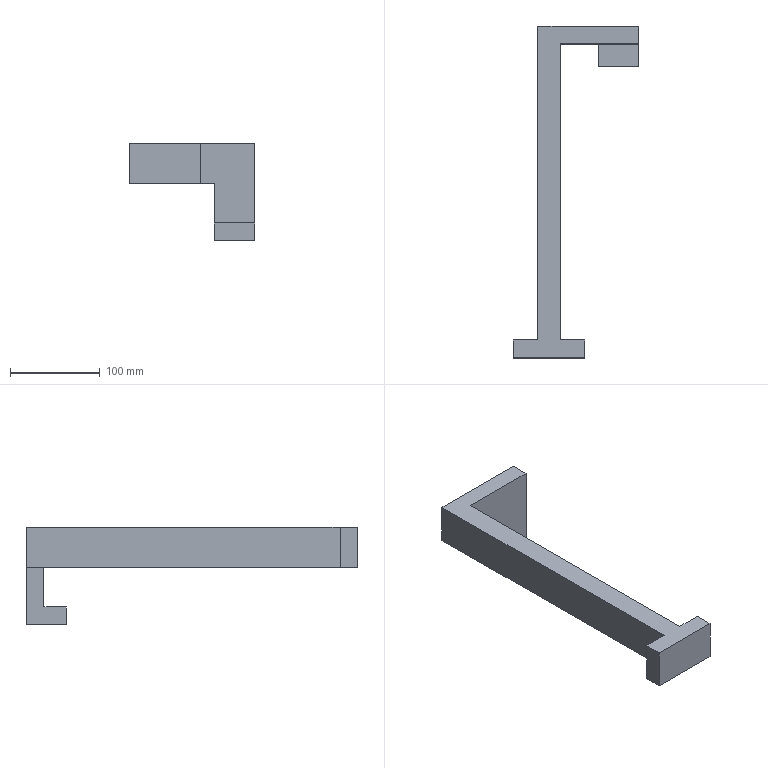Part | STEP file | Stopper | 1 solid | 16 faces | box 140 x 370 x 109 mm | volume 624600 mm3 | plane 16
STEP:
#1=CARTESIAN_POINT('',(0.,0.,0.));
#2=DIRECTION('',(0.,0.,1.));
#3=DIRECTION('',(1.,0.,0.));
#4=AXIS2_PLACEMENT_3D('',#1,#2,#3);
#5=CARTESIAN_POINT('',(112.5,-20.,-44.));
#6=VERTEX_POINT('',#5);
#7=CARTESIAN_POINT('',(67.5,-20.,-44.));
#8=VERTEX_POINT('',#7);
#9=CARTESIAN_POINT('',(67.5,-20.,-44.));
#10=DIRECTION('',(-1.,0.,0.));
#11=VECTOR('',#10,1.);
#12=LINE('',#9,#11);
#13=CARTESIAN_POINT('',(112.5,-20.,45.));
#14=DIRECTION('',(0.,1.,0.));
#15=DIRECTION('',(0.,0.,1.));
#16=AXIS2_PLACEMENT_3D('',#13,#14,#15);
#17=PLANE('',#16);
#18=CARTESIAN_POINT('',(-89.,-45.));
#19=DIRECTION('',(0.,-1.));
#20=VECTOR('',#19,1.);
#21=LINE('',#18,#20);
#22=(GEOMETRIC_REPRESENTATION_CONTEXT(2)PARAMETRIC_REPRESENTATION_CONTEXT()REPRESENTATION_CONTEXT('',''));
#23=DEFINITIONAL_REPRESENTATION('',(#21),#22);
#24=PCURVE('',#17,#23);
#25=CARTESIAN_POINT('',(67.5,-45.,-44.));
#26=DIRECTION('',(0.,0.,-1.));
#27=DIRECTION('',(-1.,0.,0.));
#28=AXIS2_PLACEMENT_3D('',#25,#26,#27);
#29=PLANE('',#28);
#30=CARTESIAN_POINT('',(0.,25.));
#31=DIRECTION('',(1.,0.));
#32=VECTOR('',#31,1.);
#33=LINE('',#30,#32);
#34=(GEOMETRIC_REPRESENTATION_CONTEXT(2)PARAMETRIC_REPRESENTATION_CONTEXT()REPRESENTATION_CONTEXT('',''));
#35=DEFINITIONAL_REPRESENTATION('',(#33),#34);
#36=PCURVE('',#29,#35);
#37=SURFACE_CURVE('',#12,(#24,#36),.PCURVE_S1.);
#38=EDGE_CURVE('',#6,#8,#37,.T.);
#39=ORIENTED_EDGE('',*,*,#38,.F.);
#40=CARTESIAN_POINT('',(112.5,-20.,45.));
#41=VERTEX_POINT('',#40);
#42=CARTESIAN_POINT('',(112.5,-20.,45.));
#43=DIRECTION('',(0.,0.,-1.));
#44=VECTOR('',#43,1.);
#45=LINE('',#42,#44);
#46=CARTESIAN_POINT('',(0.,0.));
#47=DIRECTION('',(-1.,0.));
#48=VECTOR('',#47,1.);
#49=LINE('',#46,#48);
#50=(GEOMETRIC_REPRESENTATION_CONTEXT(2)PARAMETRIC_REPRESENTATION_CONTEXT()REPRESENTATION_CONTEXT('',''));
#51=DEFINITIONAL_REPRESENTATION('',(#49),#50);
#52=PCURVE('',#17,#51);
#53=CARTESIAN_POINT('',(112.5,-20.,45.));
#54=DIRECTION('',(1.,0.,0.));
#55=DIRECTION('',(0.,0.,-1.));
#56=AXIS2_PLACEMENT_3D('',#53,#54,#55);
#57=PLANE('',#56);
#58=CARTESIAN_POINT('',(0.,0.));
#59=DIRECTION('',(1.,0.));
#60=VECTOR('',#59,1.);
#61=LINE('',#58,#60);
#62=(GEOMETRIC_REPRESENTATION_CONTEXT(2)PARAMETRIC_REPRESENTATION_CONTEXT()REPRESENTATION_CONTEXT('',''));
#63=DEFINITIONAL_REPRESENTATION('',(#61),#62);
#64=PCURVE('',#57,#63);
#65=SURFACE_CURVE('',#45,(#52,#64),.PCURVE_S1.);
#66=EDGE_CURVE('',#41,#6,#65,.T.);
#67=ORIENTED_EDGE('',*,*,#66,.F.);
#68=CARTESIAN_POINT('',(25.,-20.,45.));
#69=VERTEX_POINT('',#68);
#70=CARTESIAN_POINT('',(112.5,-20.,45.));
#71=DIRECTION('',(-1.,0.,0.));
#72=VECTOR('',#71,1.);
#73=LINE('',#70,#72);
#74=CARTESIAN_POINT('',(0.,0.));
#75=DIRECTION('',(0.,-1.));
#76=VECTOR('',#75,1.);
#77=LINE('',#74,#76);
#78=(GEOMETRIC_REPRESENTATION_CONTEXT(2)PARAMETRIC_REPRESENTATION_CONTEXT()REPRESENTATION_CONTEXT('',''));
#79=DEFINITIONAL_REPRESENTATION('',(#77),#78);
#80=PCURVE('',#17,#79);
#81=CARTESIAN_POINT('',(0.,0.,45.));
#82=DIRECTION('',(0.,0.,1.));
#83=DIRECTION('',(1.,0.,0.));
#84=AXIS2_PLACEMENT_3D('',#81,#82,#83);
#85=PLANE('',#84);
#86=CARTESIAN_POINT('',(112.5,-20.));
#87=DIRECTION('',(-1.,0.));
#88=VECTOR('',#87,1.);
#89=LINE('',#86,#88);
#90=(GEOMETRIC_REPRESENTATION_CONTEXT(2)PARAMETRIC_REPRESENTATION_CONTEXT()REPRESENTATION_CONTEXT('',''));
#91=DEFINITIONAL_REPRESENTATION('',(#89),#90);
#92=PCURVE('',#85,#91);
#93=SURFACE_CURVE('',#73,(#80,#92),.PCURVE_S1.);
#94=EDGE_CURVE('',#41,#69,#93,.T.);
#95=ORIENTED_EDGE('',*,*,#94,.T.);
#96=CARTESIAN_POINT('',(25.,-20.,0.));
#97=VERTEX_POINT('',#96);
#98=CARTESIAN_POINT('',(25.,-20.,45.));
#99=DIRECTION('',(0.,0.,-1.));
#100=VECTOR('',#99,1.);
#101=LINE('',#98,#100);
#102=CARTESIAN_POINT('',(0.,-87.5));
#103=DIRECTION('',(-1.,0.));
#104=VECTOR('',#103,1.);
#105=LINE('',#102,#104);
#106=(GEOMETRIC_REPRESENTATION_CONTEXT(2)PARAMETRIC_REPRESENTATION_CONTEXT()REPRESENTATION_CONTEXT('',''));
#107=DEFINITIONAL_REPRESENTATION('',(#105),#106);
#108=PCURVE('',#17,#107);
#109=CARTESIAN_POINT('',(25.,-350.,45.));
#110=DIRECTION('',(-1.,0.,0.));
#111=DIRECTION('',(0.,0.,1.));
#112=AXIS2_PLACEMENT_3D('',#109,#110,#111);
#113=PLANE('',#112);
#114=CARTESIAN_POINT('',(0.,330.));
#115=DIRECTION('',(-1.,0.));
#116=VECTOR('',#115,1.);
#117=LINE('',#114,#116);
#118=(GEOMETRIC_REPRESENTATION_CONTEXT(2)PARAMETRIC_REPRESENTATION_CONTEXT()REPRESENTATION_CONTEXT('',''));
#119=DEFINITIONAL_REPRESENTATION('',(#117),#118);
#120=PCURVE('',#113,#119);
#121=SURFACE_CURVE('',#101,(#108,#120),.PCURVE_S1.);
#122=EDGE_CURVE('',#69,#97,#121,.T.);
#123=ORIENTED_EDGE('',*,*,#122,.T.);
#124=CARTESIAN_POINT('',(67.5,-20.,0.));
#125=VERTEX_POINT('',#124);
#126=CARTESIAN_POINT('',(112.5,-20.,0.));
#127=DIRECTION('',(-1.,0.,0.));
#128=VECTOR('',#127,1.);
#129=LINE('',#126,#128);
#130=CARTESIAN_POINT('',(-45.,0.));
#131=DIRECTION('',(0.,-1.));
#132=VECTOR('',#131,1.);
#133=LINE('',#130,#132);
#134=(GEOMETRIC_REPRESENTATION_CONTEXT(2)PARAMETRIC_REPRESENTATION_CONTEXT()REPRESENTATION_CONTEXT('',''));
#135=DEFINITIONAL_REPRESENTATION('',(#133),#134);
#136=PCURVE('',#17,#135);
#137=CARTESIAN_POINT('',(0.,0.,0.));
#138=DIRECTION('',(0.,0.,1.));
#139=DIRECTION('',(1.,0.,0.));
#140=AXIS2_PLACEMENT_3D('',#137,#138,#139);
#141=PLANE('',#140);
#142=CARTESIAN_POINT('',(112.5,-20.));
#143=DIRECTION('',(-1.,0.));
#144=VECTOR('',#143,1.);
#145=LINE('',#142,#144);
#146=(GEOMETRIC_REPRESENTATION_CONTEXT(2)PARAMETRIC_REPRESENTATION_CONTEXT()REPRESENTATION_CONTEXT('',''));
#147=DEFINITIONAL_REPRESENTATION('',(#145),#146);
#148=PCURVE('',#141,#147);
#149=SURFACE_CURVE('',#129,(#136,#148),.PCURVE_S1.);
#150=EDGE_CURVE('',#125,#97,#149,.T.);
#151=ORIENTED_EDGE('',*,*,#150,.F.);
#152=CARTESIAN_POINT('',(67.5,-20.,-64.));
#153=DIRECTION('',(0.,0.,1.));
#154=VECTOR('',#153,1.);
#155=LINE('',#152,#154);
#156=CARTESIAN_POINT('',(-109.,-45.));
#157=DIRECTION('',(1.,0.));
#158=VECTOR('',#157,1.);
#159=LINE('',#156,#158);
#160=(GEOMETRIC_REPRESENTATION_CONTEXT(2)PARAMETRIC_REPRESENTATION_CONTEXT()REPRESENTATION_CONTEXT('',''));
#161=DEFINITIONAL_REPRESENTATION('',(#159),#160);
#162=PCURVE('',#17,#161);
#163=CARTESIAN_POINT('',(67.5,0.,-64.));
#164=DIRECTION('',(1.,0.,0.));
#165=DIRECTION('',(0.,0.,-1.));
#166=AXIS2_PLACEMENT_3D('',#163,#164,#165);
#167=PLANE('',#166);
#168=CARTESIAN_POINT('',(0.,-20.));
#169=DIRECTION('',(-1.,0.));
#170=VECTOR('',#169,1.);
#171=LINE('',#168,#170);
#172=(GEOMETRIC_REPRESENTATION_CONTEXT(2)PARAMETRIC_REPRESENTATION_CONTEXT()REPRESENTATION_CONTEXT('',''));
#173=DEFINITIONAL_REPRESENTATION('',(#171),#172);
#174=PCURVE('',#167,#173);
#175=SURFACE_CURVE('',#155,(#162,#174),.PCURVE_S1.);
#176=EDGE_CURVE('',#8,#125,#175,.T.);
#177=ORIENTED_EDGE('',*,*,#176,.F.);
#178=EDGE_LOOP('',(#39,#67,#95,#123,#151,#177));
#179=FACE_BOUND('',#178,.T.);
#180=ADVANCED_FACE('',(#179),#17,.F.);
#181=CARTESIAN_POINT('',(67.5,0.,0.));
#182=VERTEX_POINT('',#181);
#183=CARTESIAN_POINT('',(67.5,0.,0.));
#184=DIRECTION('',(0.,1.,0.));
#185=VECTOR('',#184,1.);
#186=LINE('',#183,#185);
#187=CARTESIAN_POINT('',(67.5,0.));
#188=DIRECTION('',(0.,1.));
#189=VECTOR('',#188,1.);
#190=LINE('',#187,#189);
#191=(GEOMETRIC_REPRESENTATION_CONTEXT(2)PARAMETRIC_REPRESENTATION_CONTEXT()REPRESENTATION_CONTEXT('',''));
#192=DEFINITIONAL_REPRESENTATION('',(#190),#191);
#193=PCURVE('',#141,#192);
#194=CARTESIAN_POINT('',(-64.,0.));
#195=DIRECTION('',(0.,1.));
#196=VECTOR('',#195,1.);
#197=LINE('',#194,#196);
#198=(GEOMETRIC_REPRESENTATION_CONTEXT(2)PARAMETRIC_REPRESENTATION_CONTEXT()REPRESENTATION_CONTEXT('',''));
#199=DEFINITIONAL_REPRESENTATION('',(#197),#198);
#200=PCURVE('',#167,#199);
#201=SURFACE_CURVE('',#186,(#193,#200),.PCURVE_S1.);
#202=EDGE_CURVE('',#125,#182,#201,.T.);
#203=ORIENTED_EDGE('',*,*,#202,.F.);
#204=ORIENTED_EDGE('',*,*,#150,.T.);
#205=CARTESIAN_POINT('',(25.,-350.,0.));
#206=VERTEX_POINT('',#205);
#207=CARTESIAN_POINT('',(25.,-350.,0.));
#208=DIRECTION('',(0.,1.,0.));
#209=VECTOR('',#208,1.);
#210=LINE('',#207,#209);
#211=CARTESIAN_POINT('',(25.,-350.));
#212=DIRECTION('',(0.,1.));
#213=VECTOR('',#212,1.);
#214=LINE('',#211,#213);
#215=(GEOMETRIC_REPRESENTATION_CONTEXT(2)PARAMETRIC_REPRESENTATION_CONTEXT()REPRESENTATION_CONTEXT('',''));
#216=DEFINITIONAL_REPRESENTATION('',(#214),#215);
#217=PCURVE('',#141,#216);
#218=CARTESIAN_POINT('',(-45.,0.));
#219=DIRECTION('',(0.,1.));
#220=VECTOR('',#219,1.);
#221=LINE('',#218,#220);
#222=(GEOMETRIC_REPRESENTATION_CONTEXT(2)PARAMETRIC_REPRESENTATION_CONTEXT()REPRESENTATION_CONTEXT('',''));
#223=DEFINITIONAL_REPRESENTATION('',(#221),#222);
#224=PCURVE('',#113,#223);
#225=SURFACE_CURVE('',#210,(#217,#224),.PCURVE_S1.);
#226=EDGE_CURVE('',#206,#97,#225,.T.);
#227=ORIENTED_EDGE('',*,*,#226,.F.);
#228=CARTESIAN_POINT('',(52.5,-350.,0.));
#229=VERTEX_POINT('',#228);
#230=CARTESIAN_POINT('',(52.5,-350.,0.));
#231=DIRECTION('',(-1.,0.,0.));
#232=VECTOR('',#231,1.);
#233=LINE('',#230,#232);
#234=CARTESIAN_POINT('',(52.5,-350.));
#235=DIRECTION('',(-1.,0.));
#236=VECTOR('',#235,1.);
#237=LINE('',#234,#236);
#238=(GEOMETRIC_REPRESENTATION_CONTEXT(2)PARAMETRIC_REPRESENTATION_CONTEXT()REPRESENTATION_CONTEXT('',''));
#239=DEFINITIONAL_REPRESENTATION('',(#237),#238);
#240=PCURVE('',#141,#239);
#241=CARTESIAN_POINT('',(52.5,-350.,45.));
#242=DIRECTION('',(0.,-1.,0.));
#243=DIRECTION('',(0.,0.,-1.));
#244=AXIS2_PLACEMENT_3D('',#241,#242,#243);
#245=PLANE('',#244);
#246=CARTESIAN_POINT('',(45.,0.));
#247=DIRECTION('',(0.,-1.));
#248=VECTOR('',#247,1.);
#249=LINE('',#246,#248);
#250=(GEOMETRIC_REPRESENTATION_CONTEXT(2)PARAMETRIC_REPRESENTATION_CONTEXT()REPRESENTATION_CONTEXT('',''));
#251=DEFINITIONAL_REPRESENTATION('',(#249),#250);
#252=PCURVE('',#245,#251);
#253=SURFACE_CURVE('',#233,(#240,#252),.PCURVE_S1.);
#254=EDGE_CURVE('',#229,#206,#253,.T.);
#255=ORIENTED_EDGE('',*,*,#254,.F.);
#256=CARTESIAN_POINT('',(52.5,-370.,0.));
#257=VERTEX_POINT('',#256);
#258=CARTESIAN_POINT('',(52.5,-370.,0.));
#259=DIRECTION('',(0.,1.,0.));
#260=VECTOR('',#259,1.);
#261=LINE('',#258,#260);
#262=CARTESIAN_POINT('',(52.5,-370.));
#263=DIRECTION('',(0.,1.));
#264=VECTOR('',#263,1.);
#265=LINE('',#262,#264);
#266=(GEOMETRIC_REPRESENTATION_CONTEXT(2)PARAMETRIC_REPRESENTATION_CONTEXT()REPRESENTATION_CONTEXT('',''));
#267=DEFINITIONAL_REPRESENTATION('',(#265),#266);
#268=PCURVE('',#141,#267);
#269=CARTESIAN_POINT('',(52.5,-370.,45.));
#270=DIRECTION('',(-1.,0.,0.));
#271=DIRECTION('',(0.,-1.,0.));
#272=AXIS2_PLACEMENT_3D('',#269,#270,#271);
#273=PLANE('',#272);
#274=CARTESIAN_POINT('',(0.,-45.));
#275=DIRECTION('',(-1.,0.));
#276=VECTOR('',#275,1.);
#277=LINE('',#274,#276);
#278=(GEOMETRIC_REPRESENTATION_CONTEXT(2)PARAMETRIC_REPRESENTATION_CONTEXT()REPRESENTATION_CONTEXT('',''));
#279=DEFINITIONAL_REPRESENTATION('',(#277),#278);
#280=PCURVE('',#273,#279);
#281=SURFACE_CURVE('',#261,(#268,#280),.PCURVE_S1.);
#282=EDGE_CURVE('',#257,#229,#281,.T.);
#283=ORIENTED_EDGE('',*,*,#282,.F.);
#284=CARTESIAN_POINT('',(-27.5,-370.,0.));
#285=VERTEX_POINT('',#284);
#286=CARTESIAN_POINT('',(-27.5,-370.,0.));
#287=DIRECTION('',(1.,0.,0.));
#288=VECTOR('',#287,1.);
#289=LINE('',#286,#288);
#290=CARTESIAN_POINT('',(-27.5,-370.));
#291=DIRECTION('',(1.,0.));
#292=VECTOR('',#291,1.);
#293=LINE('',#290,#292);
#294=(GEOMETRIC_REPRESENTATION_CONTEXT(2)PARAMETRIC_REPRESENTATION_CONTEXT()REPRESENTATION_CONTEXT('',''));
#295=DEFINITIONAL_REPRESENTATION('',(#293),#294);
#296=PCURVE('',#141,#295);
#297=CARTESIAN_POINT('',(-27.5,-370.,45.));
#298=DIRECTION('',(0.,1.,0.));
#299=DIRECTION('',(0.,0.,1.));
#300=AXIS2_PLACEMENT_3D('',#297,#298,#299);
#301=PLANE('',#300);
#302=CARTESIAN_POINT('',(-45.,0.));
#303=DIRECTION('',(0.,1.));
#304=VECTOR('',#303,1.);
#305=LINE('',#302,#304);
#306=(GEOMETRIC_REPRESENTATION_CONTEXT(2)PARAMETRIC_REPRESENTATION_CONTEXT()REPRESENTATION_CONTEXT('',''));
#307=DEFINITIONAL_REPRESENTATION('',(#305),#306);
#308=PCURVE('',#301,#307);
#309=SURFACE_CURVE('',#289,(#296,#308),.PCURVE_S1.);
#310=EDGE_CURVE('',#285,#257,#309,.T.);
#311=ORIENTED_EDGE('',*,*,#310,.F.);
#312=CARTESIAN_POINT('',(-27.5,-350.,0.));
#313=VERTEX_POINT('',#312);
#314=CARTESIAN_POINT('',(-27.5,-350.,0.));
#315=DIRECTION('',(0.,-1.,0.));
#316=VECTOR('',#315,1.);
#317=LINE('',#314,#316);
#318=CARTESIAN_POINT('',(-27.5,-350.));
#319=DIRECTION('',(0.,-1.));
#320=VECTOR('',#319,1.);
#321=LINE('',#318,#320);
#322=(GEOMETRIC_REPRESENTATION_CONTEXT(2)PARAMETRIC_REPRESENTATION_CONTEXT()REPRESENTATION_CONTEXT('',''));
#323=DEFINITIONAL_REPRESENTATION('',(#321),#322);
#324=PCURVE('',#141,#323);
#325=CARTESIAN_POINT('',(-27.5,-350.,45.));
#326=DIRECTION('',(1.,0.,0.));
#327=DIRECTION('',(0.,1.,0.));
#328=AXIS2_PLACEMENT_3D('',#325,#326,#327);
#329=PLANE('',#328);
#330=CARTESIAN_POINT('',(0.,-45.));
#331=DIRECTION('',(-1.,0.));
#332=VECTOR('',#331,1.);
#333=LINE('',#330,#332);
#334=(GEOMETRIC_REPRESENTATION_CONTEXT(2)PARAMETRIC_REPRESENTATION_CONTEXT()REPRESENTATION_CONTEXT('',''));
#335=DEFINITIONAL_REPRESENTATION('',(#333),#334);
#336=PCURVE('',#329,#335);
#337=SURFACE_CURVE('',#317,(#324,#336),.PCURVE_S1.);
#338=EDGE_CURVE('',#313,#285,#337,.T.);
#339=ORIENTED_EDGE('',*,*,#338,.F.);
#340=CARTESIAN_POINT('',(0.,-350.,0.));
#341=VERTEX_POINT('',#340);
#342=CARTESIAN_POINT('',(0.,-350.,0.));
#343=DIRECTION('',(-1.,0.,0.));
#344=VECTOR('',#343,1.);
#345=LINE('',#342,#344);
#346=CARTESIAN_POINT('',(0.,-350.));
#347=DIRECTION('',(-1.,0.));
#348=VECTOR('',#347,1.);
#349=LINE('',#346,#348);
#350=(GEOMETRIC_REPRESENTATION_CONTEXT(2)PARAMETRIC_REPRESENTATION_CONTEXT()REPRESENTATION_CONTEXT('',''));
#351=DEFINITIONAL_REPRESENTATION('',(#349),#350);
#352=PCURVE('',#141,#351);
#353=CARTESIAN_POINT('',(0.,-350.,45.));
#354=DIRECTION('',(0.,-1.,0.));
#355=DIRECTION('',(0.,0.,-1.));
#356=AXIS2_PLACEMENT_3D('',#353,#354,#355);
#357=PLANE('',#356);
#358=CARTESIAN_POINT('',(45.,0.));
#359=DIRECTION('',(0.,-1.));
#360=VECTOR('',#359,1.);
#361=LINE('',#358,#360);
#362=(GEOMETRIC_REPRESENTATION_CONTEXT(2)PARAMETRIC_REPRESENTATION_CONTEXT()REPRESENTATION_CONTEXT('',''));
#363=DEFINITIONAL_REPRESENTATION('',(#361),#362);
#364=PCURVE('',#357,#363);
#365=SURFACE_CURVE('',#345,(#352,#364),.PCURVE_S1.);
#366=EDGE_CURVE('',#341,#313,#365,.T.);
#367=ORIENTED_EDGE('',*,*,#366,.F.);
#368=CARTESIAN_POINT('',(0.,0.,0.));
#369=VERTEX_POINT('',#368);
#370=CARTESIAN_POINT('',(0.,0.,0.));
#371=DIRECTION('',(0.,-1.,0.));
#372=VECTOR('',#371,1.);
#373=LINE('',#370,#372);
#374=CARTESIAN_POINT('',(0.,0.));
#375=DIRECTION('',(0.,-1.));
#376=VECTOR('',#375,1.);
#377=LINE('',#374,#376);
#378=(GEOMETRIC_REPRESENTATION_CONTEXT(2)PARAMETRIC_REPRESENTATION_CONTEXT()REPRESENTATION_CONTEXT('',''));
#379=DEFINITIONAL_REPRESENTATION('',(#377),#378);
#380=PCURVE('',#141,#379);
#381=CARTESIAN_POINT('',(0.,0.,45.));
#382=DIRECTION('',(1.,0.,0.));
#383=DIRECTION('',(0.,1.,0.));
#384=AXIS2_PLACEMENT_3D('',#381,#382,#383);
#385=PLANE('',#384);
#386=CARTESIAN_POINT('',(0.,-45.));
#387=DIRECTION('',(-1.,0.));
#388=VECTOR('',#387,1.);
#389=LINE('',#386,#388);
#390=(GEOMETRIC_REPRESENTATION_CONTEXT(2)PARAMETRIC_REPRESENTATION_CONTEXT()REPRESENTATION_CONTEXT('',''));
#391=DEFINITIONAL_REPRESENTATION('',(#389),#390);
#392=PCURVE('',#385,#391);
#393=SURFACE_CURVE('',#373,(#380,#392),.PCURVE_S1.);
#394=EDGE_CURVE('',#369,#341,#393,.T.);
#395=ORIENTED_EDGE('',*,*,#394,.F.);
#396=CARTESIAN_POINT('',(25.,0.,0.));
#397=DIRECTION('',(-1.,0.,0.));
#398=VECTOR('',#397,1.);
#399=LINE('',#396,#398);
#400=CARTESIAN_POINT('',(25.,0.));
#401=DIRECTION('',(-1.,0.));
#402=VECTOR('',#401,1.);
#403=LINE('',#400,#402);
#404=(GEOMETRIC_REPRESENTATION_CONTEXT(2)PARAMETRIC_REPRESENTATION_CONTEXT()REPRESENTATION_CONTEXT('',''));
#405=DEFINITIONAL_REPRESENTATION('',(#403),#404);
#406=PCURVE('',#141,#405);
#407=CARTESIAN_POINT('',(25.,0.,45.));
#408=DIRECTION('',(0.,-1.,0.));
#409=DIRECTION('',(1.,0.,0.));
#410=AXIS2_PLACEMENT_3D('',#407,#408,#409);
#411=PLANE('',#410);
#412=CARTESIAN_POINT('',(0.,-45.));
#413=DIRECTION('',(-1.,0.));
#414=VECTOR('',#413,1.);
#415=LINE('',#412,#414);
#416=(GEOMETRIC_REPRESENTATION_CONTEXT(2)PARAMETRIC_REPRESENTATION_CONTEXT()REPRESENTATION_CONTEXT('',''));
#417=DEFINITIONAL_REPRESENTATION('',(#415),#416);
#418=PCURVE('',#411,#417);
#419=SURFACE_CURVE('',#399,(#406,#418),.PCURVE_S1.);
#420=EDGE_CURVE('',#182,#369,#419,.T.);
#421=ORIENTED_EDGE('',*,*,#420,.F.);
#422=EDGE_LOOP('',(#203,#204,#227,#255,#283,#311,#339,#367,#395,#421));
#423=FACE_BOUND('',#422,.T.);
#424=ADVANCED_FACE('',(#423),#141,.F.);
#425=ORIENTED_EDGE('',*,*,#122,.F.);
#426=CARTESIAN_POINT('',(25.,-350.,45.));
#427=VERTEX_POINT('',#426);
#428=CARTESIAN_POINT('',(25.,-350.,45.));
#429=DIRECTION('',(0.,1.,0.));
#430=VECTOR('',#429,1.);
#431=LINE('',#428,#430);
#432=CARTESIAN_POINT('',(0.,0.));
#433=DIRECTION('',(0.,1.));
#434=VECTOR('',#433,1.);
#435=LINE('',#432,#434);
#436=(GEOMETRIC_REPRESENTATION_CONTEXT(2)PARAMETRIC_REPRESENTATION_CONTEXT()REPRESENTATION_CONTEXT('',''));
#437=DEFINITIONAL_REPRESENTATION('',(#435),#436);
#438=PCURVE('',#113,#437);
#439=CARTESIAN_POINT('',(25.,-350.));
#440=DIRECTION('',(0.,1.));
#441=VECTOR('',#440,1.);
#442=LINE('',#439,#441);
#443=(GEOMETRIC_REPRESENTATION_CONTEXT(2)PARAMETRIC_REPRESENTATION_CONTEXT()REPRESENTATION_CONTEXT('',''));
#444=DEFINITIONAL_REPRESENTATION('',(#442),#443);
#445=PCURVE('',#85,#444);
#446=SURFACE_CURVE('',#431,(#438,#445),.PCURVE_S1.);
#447=EDGE_CURVE('',#427,#69,#446,.T.);
#448=ORIENTED_EDGE('',*,*,#447,.F.);
#449=CARTESIAN_POINT('',(25.,-350.,45.));
#450=DIRECTION('',(0.,0.,-1.));
#451=VECTOR('',#450,1.);
#452=LINE('',#449,#451);
#453=CARTESIAN_POINT('',(0.,0.));
#454=DIRECTION('',(-1.,0.));
#455=VECTOR('',#454,1.);
#456=LINE('',#453,#455);
#457=(GEOMETRIC_REPRESENTATION_CONTEXT(2)PARAMETRIC_REPRESENTATION_CONTEXT()REPRESENTATION_CONTEXT('',''));
#458=DEFINITIONAL_REPRESENTATION('',(#456),#457);
#459=PCURVE('',#113,#458);
#460=CARTESIAN_POINT('',(0.,-27.5));
#461=DIRECTION('',(1.,0.));
#462=VECTOR('',#461,1.);
#463=LINE('',#460,#462);
#464=(GEOMETRIC_REPRESENTATION_CONTEXT(2)PARAMETRIC_REPRESENTATION_CONTEXT()REPRESENTATION_CONTEXT('',''));
#465=DEFINITIONAL_REPRESENTATION('',(#463),#464);
#466=PCURVE('',#245,#465);
#467=SURFACE_CURVE('',#452,(#459,#466),.PCURVE_S1.);
#468=EDGE_CURVE('',#427,#206,#467,.T.);
#469=ORIENTED_EDGE('',*,*,#468,.T.);
#470=ORIENTED_EDGE('',*,*,#226,.T.);
#471=EDGE_LOOP('',(#425,#448,#469,#470));
#472=FACE_BOUND('',#471,.T.);
#473=ADVANCED_FACE('',(#472),#113,.F.);
#474=CARTESIAN_POINT('',(112.5,0.,-64.));
#475=VERTEX_POINT('',#474);
#476=CARTESIAN_POINT('',(112.5,0.,45.));
#477=VERTEX_POINT('',#476);
#478=CARTESIAN_POINT('',(112.5,0.,45.));
#479=DIRECTION('',(0.,0.,1.));
#480=VECTOR('',#479,1.);
#481=LINE('',#478,#480);
#482=CARTESIAN_POINT('',(87.5,0.));
#483=DIRECTION('',(0.,1.));
#484=VECTOR('',#483,1.);
#485=LINE('',#482,#484);
#486=(GEOMETRIC_REPRESENTATION_CONTEXT(2)PARAMETRIC_REPRESENTATION_CONTEXT()REPRESENTATION_CONTEXT('',''));
#487=DEFINITIONAL_REPRESENTATION('',(#485),#486);
#488=PCURVE('',#411,#487);
#489=CARTESIAN_POINT('',(0.,20.));
#490=DIRECTION('',(-1.,0.));
#491=VECTOR('',#490,1.);
#492=LINE('',#489,#491);
#493=(GEOMETRIC_REPRESENTATION_CONTEXT(2)PARAMETRIC_REPRESENTATION_CONTEXT()REPRESENTATION_CONTEXT('',''));
#494=DEFINITIONAL_REPRESENTATION('',(#492),#493);
#495=PCURVE('',#57,#494);
#496=SURFACE_CURVE('',#481,(#488,#495),.PCURVE_S1.);
#497=EDGE_CURVE('',#475,#477,#496,.T.);
#498=ORIENTED_EDGE('',*,*,#497,.F.);
#499=CARTESIAN_POINT('',(67.5,0.,-64.));
#500=VERTEX_POINT('',#499);
#501=CARTESIAN_POINT('',(112.5,0.,-64.));
#502=DIRECTION('',(1.,0.,0.));
#503=VECTOR('',#502,1.);
#504=LINE('',#501,#503);
#505=CARTESIAN_POINT('',(87.5,-109.));
#506=DIRECTION('',(1.,0.));
#507=VECTOR('',#506,1.);
#508=LINE('',#505,#507);
#509=(GEOMETRIC_REPRESENTATION_CONTEXT(2)PARAMETRIC_REPRESENTATION_CONTEXT()REPRESENTATION_CONTEXT('',''));
#510=DEFINITIONAL_REPRESENTATION('',(#508),#509);
#511=PCURVE('',#411,#510);
#512=CARTESIAN_POINT('',(112.5,-20.,-64.));
#513=DIRECTION('',(0.,0.,-1.));
#514=DIRECTION('',(-1.,0.,0.));
#515=AXIS2_PLACEMENT_3D('',#512,#513,#514);
#516=PLANE('',#515);
#517=CARTESIAN_POINT('',(0.,20.));
#518=DIRECTION('',(-1.,0.));
#519=VECTOR('',#518,1.);
#520=LINE('',#517,#519);
#521=(GEOMETRIC_REPRESENTATION_CONTEXT(2)PARAMETRIC_REPRESENTATION_CONTEXT()REPRESENTATION_CONTEXT('',''));
#522=DEFINITIONAL_REPRESENTATION('',(#520),#521);
#523=PCURVE('',#516,#522);
#524=SURFACE_CURVE('',#504,(#511,#523),.PCURVE_S1.);
#525=EDGE_CURVE('',#500,#475,#524,.T.);
#526=ORIENTED_EDGE('',*,*,#525,.F.);
#527=CARTESIAN_POINT('',(67.5,0.,-64.));
#528=DIRECTION('',(0.,0.,1.));
#529=VECTOR('',#528,1.);
#530=LINE('',#527,#529);
#531=CARTESIAN_POINT('',(42.5,-109.));
#532=DIRECTION('',(0.,1.));
#533=VECTOR('',#532,1.);
#534=LINE('',#531,#533);
#535=(GEOMETRIC_REPRESENTATION_CONTEXT(2)PARAMETRIC_REPRESENTATION_CONTEXT()REPRESENTATION_CONTEXT('',''));
#536=DEFINITIONAL_REPRESENTATION('',(#534),#535);
#537=PCURVE('',#411,#536);
#538=CARTESIAN_POINT('',(0.,0.));
#539=DIRECTION('',(-1.,0.));
#540=VECTOR('',#539,1.);
#541=LINE('',#538,#540);
#542=(GEOMETRIC_REPRESENTATION_CONTEXT(2)PARAMETRIC_REPRESENTATION_CONTEXT()REPRESENTATION_CONTEXT('',''));
#543=DEFINITIONAL_REPRESENTATION('',(#541),#542);
#544=PCURVE('',#167,#543);
#545=SURFACE_CURVE('',#530,(#537,#544),.PCURVE_S1.);
#546=EDGE_CURVE('',#500,#182,#545,.T.);
#547=ORIENTED_EDGE('',*,*,#546,.T.);
#548=ORIENTED_EDGE('',*,*,#420,.T.);
#549=CARTESIAN_POINT('',(0.,0.,45.));
#550=VERTEX_POINT('',#549);
#551=CARTESIAN_POINT('',(0.,0.,45.));
#552=DIRECTION('',(0.,0.,-1.));
#553=VECTOR('',#552,1.);
#554=LINE('',#551,#553);
#555=CARTESIAN_POINT('',(-25.,0.));
#556=DIRECTION('',(0.,-1.));
#557=VECTOR('',#556,1.);
#558=LINE('',#555,#557);
#559=(GEOMETRIC_REPRESENTATION_CONTEXT(2)PARAMETRIC_REPRESENTATION_CONTEXT()REPRESENTATION_CONTEXT('',''));
#560=DEFINITIONAL_REPRESENTATION('',(#558),#559);
#561=PCURVE('',#411,#560);
#562=CARTESIAN_POINT('',(0.,0.));
#563=DIRECTION('',(0.,-1.));
#564=VECTOR('',#563,1.);
#565=LINE('',#562,#564);
#566=(GEOMETRIC_REPRESENTATION_CONTEXT(2)PARAMETRIC_REPRESENTATION_CONTEXT()REPRESENTATION_CONTEXT('',''));
#567=DEFINITIONAL_REPRESENTATION('',(#565),#566);
#568=PCURVE('',#385,#567);
#569=SURFACE_CURVE('',#554,(#561,#568),.PCURVE_S1.);
#570=EDGE_CURVE('',#550,#369,#569,.T.);
#571=ORIENTED_EDGE('',*,*,#570,.F.);
#572=CARTESIAN_POINT('',(25.,0.,45.));
#573=DIRECTION('',(-1.,0.,0.));
#574=VECTOR('',#573,1.);
#575=LINE('',#572,#574);
#576=CARTESIAN_POINT('',(0.,0.));
#577=DIRECTION('',(-1.,0.));
#578=VECTOR('',#577,1.);
#579=LINE('',#576,#578);
#580=(GEOMETRIC_REPRESENTATION_CONTEXT(2)PARAMETRIC_REPRESENTATION_CONTEXT()REPRESENTATION_CONTEXT('',''));
#581=DEFINITIONAL_REPRESENTATION('',(#579),#580);
#582=PCURVE('',#411,#581);
#583=CARTESIAN_POINT('',(25.,0.));
#584=DIRECTION('',(-1.,0.));
#585=VECTOR('',#584,1.);
#586=LINE('',#583,#585);
#587=(GEOMETRIC_REPRESENTATION_CONTEXT(2)PARAMETRIC_REPRESENTATION_CONTEXT()REPRESENTATION_CONTEXT('',''));
#588=DEFINITIONAL_REPRESENTATION('',(#586),#587);
#589=PCURVE('',#85,#588);
#590=SURFACE_CURVE('',#575,(#582,#589),.PCURVE_S1.);
#591=EDGE_CURVE('',#477,#550,#590,.T.);
#592=ORIENTED_EDGE('',*,*,#591,.F.);
#593=EDGE_LOOP('',(#498,#526,#547,#548,#571,#592));
#594=FACE_BOUND('',#593,.T.);
#595=ADVANCED_FACE('',(#594),#411,.F.);
#596=ORIENTED_EDGE('',*,*,#394,.T.);
#597=CARTESIAN_POINT('',(0.,-350.,45.));
#598=VERTEX_POINT('',#597);
#599=CARTESIAN_POINT('',(0.,-350.,45.));
#600=DIRECTION('',(0.,0.,-1.));
#601=VECTOR('',#600,1.);
#602=LINE('',#599,#601);
#603=CARTESIAN_POINT('',(-350.,0.));
#604=DIRECTION('',(0.,-1.));
#605=VECTOR('',#604,1.);
#606=LINE('',#603,#605);
#607=(GEOMETRIC_REPRESENTATION_CONTEXT(2)PARAMETRIC_REPRESENTATION_CONTEXT()REPRESENTATION_CONTEXT('',''));
#608=DEFINITIONAL_REPRESENTATION('',(#606),#607);
#609=PCURVE('',#385,#608);
#610=CARTESIAN_POINT('',(0.,0.));
#611=DIRECTION('',(1.,0.));
#612=VECTOR('',#611,1.);
#613=LINE('',#610,#612);
#614=(GEOMETRIC_REPRESENTATION_CONTEXT(2)PARAMETRIC_REPRESENTATION_CONTEXT()REPRESENTATION_CONTEXT('',''));
#615=DEFINITIONAL_REPRESENTATION('',(#613),#614);
#616=PCURVE('',#357,#615);
#617=SURFACE_CURVE('',#602,(#609,#616),.PCURVE_S1.);
#618=EDGE_CURVE('',#598,#341,#617,.T.);
#619=ORIENTED_EDGE('',*,*,#618,.F.);
#620=CARTESIAN_POINT('',(0.,0.,45.));
#621=DIRECTION('',(0.,-1.,0.));
#622=VECTOR('',#621,1.);
#623=LINE('',#620,#622);
#624=CARTESIAN_POINT('',(0.,0.));
#625=DIRECTION('',(-1.,0.));
#626=VECTOR('',#625,1.);
#627=LINE('',#624,#626);
#628=(GEOMETRIC_REPRESENTATION_CONTEXT(2)PARAMETRIC_REPRESENTATION_CONTEXT()REPRESENTATION_CONTEXT('',''));
#629=DEFINITIONAL_REPRESENTATION('',(#627),#628);
#630=PCURVE('',#385,#629);
#631=CARTESIAN_POINT('',(0.,0.));
#632=DIRECTION('',(0.,-1.));
#633=VECTOR('',#632,1.);
#634=LINE('',#631,#633);
#635=(GEOMETRIC_REPRESENTATION_CONTEXT(2)PARAMETRIC_REPRESENTATION_CONTEXT()REPRESENTATION_CONTEXT('',''));
#636=DEFINITIONAL_REPRESENTATION('',(#634),#635);
#637=PCURVE('',#85,#636);
#638=SURFACE_CURVE('',#623,(#630,#637),.PCURVE_S1.);
#639=EDGE_CURVE('',#550,#598,#638,.T.);
#640=ORIENTED_EDGE('',*,*,#639,.F.);
#641=ORIENTED_EDGE('',*,*,#570,.T.);
#642=EDGE_LOOP('',(#596,#619,#640,#641));
#643=FACE_BOUND('',#642,.T.);
#644=ADVANCED_FACE('',(#643),#385,.F.);
#645=ORIENTED_EDGE('',*,*,#366,.T.);
#646=CARTESIAN_POINT('',(-27.5,-350.,45.));
#647=VERTEX_POINT('',#646);
#648=CARTESIAN_POINT('',(-27.5,-350.,45.));
#649=DIRECTION('',(0.,0.,-1.));
#650=VECTOR('',#649,1.);
#651=LINE('',#648,#650);
#652=CARTESIAN_POINT('',(0.,-27.5));
#653=DIRECTION('',(1.,0.));
#654=VECTOR('',#653,1.);
#655=LINE('',#652,#654);
#656=(GEOMETRIC_REPRESENTATION_CONTEXT(2)PARAMETRIC_REPRESENTATION_CONTEXT()REPRESENTATION_CONTEXT('',''));
#657=DEFINITIONAL_REPRESENTATION('',(#655),#656);
#658=PCURVE('',#357,#657);
#659=CARTESIAN_POINT('',(0.,0.));
#660=DIRECTION('',(0.,-1.));
#661=VECTOR('',#660,1.);
#662=LINE('',#659,#661);
#663=(GEOMETRIC_REPRESENTATION_CONTEXT(2)PARAMETRIC_REPRESENTATION_CONTEXT()REPRESENTATION_CONTEXT('',''));
#664=DEFINITIONAL_REPRESENTATION('',(#662),#663);
#665=PCURVE('',#329,#664);
#666=SURFACE_CURVE('',#651,(#658,#665),.PCURVE_S1.);
#667=EDGE_CURVE('',#647,#313,#666,.T.);
#668=ORIENTED_EDGE('',*,*,#667,.F.);
#669=CARTESIAN_POINT('',(0.,-350.,45.));
#670=DIRECTION('',(-1.,0.,0.));
#671=VECTOR('',#670,1.);
#672=LINE('',#669,#671);
#673=CARTESIAN_POINT('',(0.,0.));
#674=DIRECTION('',(0.,-1.));
#675=VECTOR('',#674,1.);
#676=LINE('',#673,#675);
#677=(GEOMETRIC_REPRESENTATION_CONTEXT(2)PARAMETRIC_REPRESENTATION_CONTEXT()REPRESENTATION_CONTEXT('',''));
#678=DEFINITIONAL_REPRESENTATION('',(#676),#677);
#679=PCURVE('',#357,#678);
#680=CARTESIAN_POINT('',(0.,-350.));
#681=DIRECTION('',(-1.,0.));
#682=VECTOR('',#681,1.);
#683=LINE('',#680,#682);
#684=(GEOMETRIC_REPRESENTATION_CONTEXT(2)PARAMETRIC_REPRESENTATION_CONTEXT()REPRESENTATION_CONTEXT('',''));
#685=DEFINITIONAL_REPRESENTATION('',(#683),#684);
#686=PCURVE('',#85,#685);
#687=SURFACE_CURVE('',#672,(#679,#686),.PCURVE_S1.);
#688=EDGE_CURVE('',#598,#647,#687,.T.);
#689=ORIENTED_EDGE('',*,*,#688,.F.);
#690=ORIENTED_EDGE('',*,*,#618,.T.);
#691=EDGE_LOOP('',(#645,#668,#689,#690));
#692=FACE_BOUND('',#691,.T.);
#693=ADVANCED_FACE('',(#692),#357,.F.);
#694=ORIENTED_EDGE('',*,*,#338,.T.);
#695=CARTESIAN_POINT('',(-27.5,-370.,45.));
#696=VERTEX_POINT('',#695);
#697=CARTESIAN_POINT('',(-27.5,-370.,45.));
#698=DIRECTION('',(0.,0.,-1.));
#699=VECTOR('',#698,1.);
#700=LINE('',#697,#699);
#701=CARTESIAN_POINT('',(-20.,0.));
#702=DIRECTION('',(0.,-1.));
#703=VECTOR('',#702,1.);
#704=LINE('',#701,#703);
#705=(GEOMETRIC_REPRESENTATION_CONTEXT(2)PARAMETRIC_REPRESENTATION_CONTEXT()REPRESENTATION_CONTEXT('',''));
#706=DEFINITIONAL_REPRESENTATION('',(#704),#705);
#707=PCURVE('',#329,#706);
#708=CARTESIAN_POINT('',(0.,0.));
#709=DIRECTION('',(-1.,0.));
#710=VECTOR('',#709,1.);
#711=LINE('',#708,#710);
#712=(GEOMETRIC_REPRESENTATION_CONTEXT(2)PARAMETRIC_REPRESENTATION_CONTEXT()REPRESENTATION_CONTEXT('',''));
#713=DEFINITIONAL_REPRESENTATION('',(#711),#712);
#714=PCURVE('',#301,#713);
#715=SURFACE_CURVE('',#700,(#707,#714),.PCURVE_S1.);
#716=EDGE_CURVE('',#696,#285,#715,.T.);
#717=ORIENTED_EDGE('',*,*,#716,.F.);
#718=CARTESIAN_POINT('',(-27.5,-350.,45.));
#719=DIRECTION('',(0.,-1.,0.));
#720=VECTOR('',#719,1.);
#721=LINE('',#718,#720);
#722=CARTESIAN_POINT('',(0.,0.));
#723=DIRECTION('',(-1.,0.));
#724=VECTOR('',#723,1.);
#725=LINE('',#722,#724);
#726=(GEOMETRIC_REPRESENTATION_CONTEXT(2)PARAMETRIC_REPRESENTATION_CONTEXT()REPRESENTATION_CONTEXT('',''));
#727=DEFINITIONAL_REPRESENTATION('',(#725),#726);
#728=PCURVE('',#329,#727);
#729=CARTESIAN_POINT('',(-27.5,-350.));
#730=DIRECTION('',(0.,-1.));
#731=VECTOR('',#730,1.);
#732=LINE('',#729,#731);
#733=(GEOMETRIC_REPRESENTATION_CONTEXT(2)PARAMETRIC_REPRESENTATION_CONTEXT()REPRESENTATION_CONTEXT('',''));
#734=DEFINITIONAL_REPRESENTATION('',(#732),#733);
#735=PCURVE('',#85,#734);
#736=SURFACE_CURVE('',#721,(#728,#735),.PCURVE_S1.);
#737=EDGE_CURVE('',#647,#696,#736,.T.);
#738=ORIENTED_EDGE('',*,*,#737,.F.);
#739=ORIENTED_EDGE('',*,*,#667,.T.);
#740=EDGE_LOOP('',(#694,#717,#738,#739));
#741=FACE_BOUND('',#740,.T.);
#742=ADVANCED_FACE('',(#741),#329,.F.);
#743=ORIENTED_EDGE('',*,*,#310,.T.);
#744=CARTESIAN_POINT('',(52.5,-370.,45.));
#745=VERTEX_POINT('',#744);
#746=CARTESIAN_POINT('',(52.5,-370.,45.));
#747=DIRECTION('',(0.,0.,-1.));
#748=VECTOR('',#747,1.);
#749=LINE('',#746,#748);
#750=CARTESIAN_POINT('',(0.,80.));
#751=DIRECTION('',(-1.,0.));
#752=VECTOR('',#751,1.);
#753=LINE('',#750,#752);
#754=(GEOMETRIC_REPRESENTATION_CONTEXT(2)PARAMETRIC_REPRESENTATION_CONTEXT()REPRESENTATION_CONTEXT('',''));
#755=DEFINITIONAL_REPRESENTATION('',(#753),#754);
#756=PCURVE('',#301,#755);
#757=CARTESIAN_POINT('',(0.,0.));
#758=DIRECTION('',(0.,-1.));
#759=VECTOR('',#758,1.);
#760=LINE('',#757,#759);
#761=(GEOMETRIC_REPRESENTATION_CONTEXT(2)PARAMETRIC_REPRESENTATION_CONTEXT()REPRESENTATION_CONTEXT('',''));
#762=DEFINITIONAL_REPRESENTATION('',(#760),#761);
#763=PCURVE('',#273,#762);
#764=SURFACE_CURVE('',#749,(#756,#763),.PCURVE_S1.);
#765=EDGE_CURVE('',#745,#257,#764,.T.);
#766=ORIENTED_EDGE('',*,*,#765,.F.);
#767=CARTESIAN_POINT('',(-27.5,-370.,45.));
#768=DIRECTION('',(1.,0.,0.));
#769=VECTOR('',#768,1.);
#770=LINE('',#767,#769);
#771=CARTESIAN_POINT('',(0.,0.));
#772=DIRECTION('',(0.,1.));
#773=VECTOR('',#772,1.);
#774=LINE('',#771,#773);
#775=(GEOMETRIC_REPRESENTATION_CONTEXT(2)PARAMETRIC_REPRESENTATION_CONTEXT()REPRESENTATION_CONTEXT('',''));
#776=DEFINITIONAL_REPRESENTATION('',(#774),#775);
#777=PCURVE('',#301,#776);
#778=CARTESIAN_POINT('',(-27.5,-370.));
#779=DIRECTION('',(1.,0.));
#780=VECTOR('',#779,1.);
#781=LINE('',#778,#780);
#782=(GEOMETRIC_REPRESENTATION_CONTEXT(2)PARAMETRIC_REPRESENTATION_CONTEXT()REPRESENTATION_CONTEXT('',''));
#783=DEFINITIONAL_REPRESENTATION('',(#781),#782);
#784=PCURVE('',#85,#783);
#785=SURFACE_CURVE('',#770,(#777,#784),.PCURVE_S1.);
#786=EDGE_CURVE('',#696,#745,#785,.T.);
#787=ORIENTED_EDGE('',*,*,#786,.F.);
#788=ORIENTED_EDGE('',*,*,#716,.T.);
#789=EDGE_LOOP('',(#743,#766,#787,#788));
#790=FACE_BOUND('',#789,.T.);
#791=ADVANCED_FACE('',(#790),#301,.F.);
#792=ORIENTED_EDGE('',*,*,#282,.T.);
#793=CARTESIAN_POINT('',(52.5,-350.,45.));
#794=VERTEX_POINT('',#793);
#795=CARTESIAN_POINT('',(52.5,-350.,45.));
#796=DIRECTION('',(0.,0.,-1.));
#797=VECTOR('',#796,1.);
#798=LINE('',#795,#797);
#799=CARTESIAN_POINT('',(-20.,0.));
#800=DIRECTION('',(0.,-1.));
#801=VECTOR('',#800,1.);
#802=LINE('',#799,#801);
#803=(GEOMETRIC_REPRESENTATION_CONTEXT(2)PARAMETRIC_REPRESENTATION_CONTEXT()REPRESENTATION_CONTEXT('',''));
#804=DEFINITIONAL_REPRESENTATION('',(#802),#803);
#805=PCURVE('',#273,#804);
#806=CARTESIAN_POINT('',(0.,0.));
#807=DIRECTION('',(1.,0.));
#808=VECTOR('',#807,1.);
#809=LINE('',#806,#808);
#810=(GEOMETRIC_REPRESENTATION_CONTEXT(2)PARAMETRIC_REPRESENTATION_CONTEXT()REPRESENTATION_CONTEXT('',''));
#811=DEFINITIONAL_REPRESENTATION('',(#809),#810);
#812=PCURVE('',#245,#811);
#813=SURFACE_CURVE('',#798,(#805,#812),.PCURVE_S1.);
#814=EDGE_CURVE('',#794,#229,#813,.T.);
#815=ORIENTED_EDGE('',*,*,#814,.F.);
#816=CARTESIAN_POINT('',(52.5,-370.,45.));
#817=DIRECTION('',(0.,1.,0.));
#818=VECTOR('',#817,1.);
#819=LINE('',#816,#818);
#820=CARTESIAN_POINT('',(0.,0.));
#821=DIRECTION('',(-1.,0.));
#822=VECTOR('',#821,1.);
#823=LINE('',#820,#822);
#824=(GEOMETRIC_REPRESENTATION_CONTEXT(2)PARAMETRIC_REPRESENTATION_CONTEXT()REPRESENTATION_CONTEXT('',''));
#825=DEFINITIONAL_REPRESENTATION('',(#823),#824);
#826=PCURVE('',#273,#825);
#827=CARTESIAN_POINT('',(52.5,-370.));
#828=DIRECTION('',(0.,1.));
#829=VECTOR('',#828,1.);
#830=LINE('',#827,#829);
#831=(GEOMETRIC_REPRESENTATION_CONTEXT(2)PARAMETRIC_REPRESENTATION_CONTEXT()REPRESENTATION_CONTEXT('',''));
#832=DEFINITIONAL_REPRESENTATION('',(#830),#831);
#833=PCURVE('',#85,#832);
#834=SURFACE_CURVE('',#819,(#826,#833),.PCURVE_S1.);
#835=EDGE_CURVE('',#745,#794,#834,.T.);
#836=ORIENTED_EDGE('',*,*,#835,.F.);
#837=ORIENTED_EDGE('',*,*,#765,.T.);
#838=EDGE_LOOP('',(#792,#815,#836,#837));
#839=FACE_BOUND('',#838,.T.);
#840=ADVANCED_FACE('',(#839),#273,.F.);
#841=ORIENTED_EDGE('',*,*,#254,.T.);
#842=ORIENTED_EDGE('',*,*,#468,.F.);
#843=CARTESIAN_POINT('',(52.5,-350.,45.));
#844=DIRECTION('',(-1.,0.,0.));
#845=VECTOR('',#844,1.);
#846=LINE('',#843,#845);
#847=CARTESIAN_POINT('',(0.,0.));
#848=DIRECTION('',(0.,-1.));
#849=VECTOR('',#848,1.);
#850=LINE('',#847,#849);
#851=(GEOMETRIC_REPRESENTATION_CONTEXT(2)PARAMETRIC_REPRESENTATION_CONTEXT()REPRESENTATION_CONTEXT('',''));
#852=DEFINITIONAL_REPRESENTATION('',(#850),#851);
#853=PCURVE('',#245,#852);
#854=CARTESIAN_POINT('',(52.5,-350.));
#855=DIRECTION('',(-1.,0.));
#856=VECTOR('',#855,1.);
#857=LINE('',#854,#856);
#858=(GEOMETRIC_REPRESENTATION_CONTEXT(2)PARAMETRIC_REPRESENTATION_CONTEXT()REPRESENTATION_CONTEXT('',''));
#859=DEFINITIONAL_REPRESENTATION('',(#857),#858);
#860=PCURVE('',#85,#859);
#861=SURFACE_CURVE('',#846,(#853,#860),.PCURVE_S1.);
#862=EDGE_CURVE('',#794,#427,#861,.T.);
#863=ORIENTED_EDGE('',*,*,#862,.F.);
#864=ORIENTED_EDGE('',*,*,#814,.T.);
#865=EDGE_LOOP('',(#841,#842,#863,#864));
#866=FACE_BOUND('',#865,.T.);
#867=ADVANCED_FACE('',(#866),#245,.F.);
#868=ORIENTED_EDGE('',*,*,#591,.T.);
#869=ORIENTED_EDGE('',*,*,#639,.T.);
#870=ORIENTED_EDGE('',*,*,#688,.T.);
#871=ORIENTED_EDGE('',*,*,#737,.T.);
#872=ORIENTED_EDGE('',*,*,#786,.T.);
#873=ORIENTED_EDGE('',*,*,#835,.T.);
#874=ORIENTED_EDGE('',*,*,#862,.T.);
#875=ORIENTED_EDGE('',*,*,#447,.T.);
#876=ORIENTED_EDGE('',*,*,#94,.F.);
#877=CARTESIAN_POINT('',(112.5,0.,45.));
#878=DIRECTION('',(0.,-1.,0.));
#879=VECTOR('',#878,1.);
#880=LINE('',#877,#879);
#881=CARTESIAN_POINT('',(112.5,0.));
#882=DIRECTION('',(0.,-1.));
#883=VECTOR('',#882,1.);
#884=LINE('',#881,#883);
#885=(GEOMETRIC_REPRESENTATION_CONTEXT(2)PARAMETRIC_REPRESENTATION_CONTEXT()REPRESENTATION_CONTEXT('',''));
#886=DEFINITIONAL_REPRESENTATION('',(#884),#885);
#887=PCURVE('',#85,#886);
#888=CARTESIAN_POINT('',(0.,20.));
#889=DIRECTION('',(0.,-1.));
#890=VECTOR('',#889,1.);
#891=LINE('',#888,#890);
#892=(GEOMETRIC_REPRESENTATION_CONTEXT(2)PARAMETRIC_REPRESENTATION_CONTEXT()REPRESENTATION_CONTEXT('',''));
#893=DEFINITIONAL_REPRESENTATION('',(#891),#892);
#894=PCURVE('',#57,#893);
#895=SURFACE_CURVE('',#880,(#887,#894),.PCURVE_S1.);
#896=EDGE_CURVE('',#477,#41,#895,.T.);
#897=ORIENTED_EDGE('',*,*,#896,.F.);
#898=EDGE_LOOP('',(#868,#869,#870,#871,#872,#873,#874,#875,#876,#897));
#899=FACE_BOUND('',#898,.T.);
#900=ADVANCED_FACE('',(#899),#85,.T.);
#901=ORIENTED_EDGE('',*,*,#896,.T.);
#902=ORIENTED_EDGE('',*,*,#66,.T.);
#903=CARTESIAN_POINT('',(112.5,-45.,-44.));
#904=VERTEX_POINT('',#903);
#905=CARTESIAN_POINT('',(112.5,-45.,-44.));
#906=DIRECTION('',(0.,1.,0.));
#907=VECTOR('',#906,1.);
#908=LINE('',#905,#907);
#909=CARTESIAN_POINT('',(89.,-25.));
#910=DIRECTION('',(0.,1.));
#911=VECTOR('',#910,1.);
#912=LINE('',#909,#911);
#913=(GEOMETRIC_REPRESENTATION_CONTEXT(2)PARAMETRIC_REPRESENTATION_CONTEXT()REPRESENTATION_CONTEXT('',''));
#914=DEFINITIONAL_REPRESENTATION('',(#912),#913);
#915=PCURVE('',#57,#914);
#916=CARTESIAN_POINT('',(-45.,0.));
#917=DIRECTION('',(0.,1.));
#918=VECTOR('',#917,1.);
#919=LINE('',#916,#918);
#920=(GEOMETRIC_REPRESENTATION_CONTEXT(2)PARAMETRIC_REPRESENTATION_CONTEXT()REPRESENTATION_CONTEXT('',''));
#921=DEFINITIONAL_REPRESENTATION('',(#919),#920);
#922=PCURVE('',#29,#921);
#923=SURFACE_CURVE('',#908,(#915,#922),.PCURVE_S1.);
#924=EDGE_CURVE('',#904,#6,#923,.T.);
#925=ORIENTED_EDGE('',*,*,#924,.F.);
#926=CARTESIAN_POINT('',(112.5,-45.,-64.));
#927=VERTEX_POINT('',#926);
#928=CARTESIAN_POINT('',(112.5,-45.,-64.));
#929=DIRECTION('',(0.,0.,1.));
#930=VECTOR('',#929,1.);
#931=LINE('',#928,#930);
#932=CARTESIAN_POINT('',(109.,-25.));
#933=DIRECTION('',(-1.,0.));
#934=VECTOR('',#933,1.);
#935=LINE('',#932,#934);
#936=(GEOMETRIC_REPRESENTATION_CONTEXT(2)PARAMETRIC_REPRESENTATION_CONTEXT()REPRESENTATION_CONTEXT('',''));
#937=DEFINITIONAL_REPRESENTATION('',(#935),#936);
#938=PCURVE('',#57,#937);
#939=CARTESIAN_POINT('',(67.5,-45.,-44.));
#940=DIRECTION('',(0.,1.,0.));
#941=DIRECTION('',(0.,0.,1.));
#942=AXIS2_PLACEMENT_3D('',#939,#940,#941);
#943=PLANE('',#942);
#944=CARTESIAN_POINT('',(-20.,45.));
#945=DIRECTION('',(1.,0.));
#946=VECTOR('',#945,1.);
#947=LINE('',#944,#946);
#948=(GEOMETRIC_REPRESENTATION_CONTEXT(2)PARAMETRIC_REPRESENTATION_CONTEXT()REPRESENTATION_CONTEXT('',''));
#949=DEFINITIONAL_REPRESENTATION('',(#947),#948);
#950=PCURVE('',#943,#949);
#951=SURFACE_CURVE('',#931,(#938,#950),.PCURVE_S1.);
#952=EDGE_CURVE('',#927,#904,#951,.T.);
#953=ORIENTED_EDGE('',*,*,#952,.F.);
#954=CARTESIAN_POINT('',(112.5,0.,-64.));
#955=DIRECTION('',(0.,-1.,0.));
#956=VECTOR('',#955,1.);
#957=LINE('',#954,#956);
#958=CARTESIAN_POINT('',(109.,20.));
#959=DIRECTION('',(0.,-1.));
#960=VECTOR('',#959,1.);
#961=LINE('',#958,#960);
#962=(GEOMETRIC_REPRESENTATION_CONTEXT(2)PARAMETRIC_REPRESENTATION_CONTEXT()REPRESENTATION_CONTEXT('',''));
#963=DEFINITIONAL_REPRESENTATION('',(#961),#962);
#964=PCURVE('',#57,#963);
#965=CARTESIAN_POINT('',(0.,20.));
#966=DIRECTION('',(0.,-1.));
#967=VECTOR('',#966,1.);
#968=LINE('',#965,#967);
#969=(GEOMETRIC_REPRESENTATION_CONTEXT(2)PARAMETRIC_REPRESENTATION_CONTEXT()REPRESENTATION_CONTEXT('',''));
#970=DEFINITIONAL_REPRESENTATION('',(#968),#969);
#971=PCURVE('',#516,#970);
#972=SURFACE_CURVE('',#957,(#964,#971),.PCURVE_S1.);
#973=EDGE_CURVE('',#475,#927,#972,.T.);
#974=ORIENTED_EDGE('',*,*,#973,.F.);
#975=ORIENTED_EDGE('',*,*,#497,.T.);
#976=EDGE_LOOP('',(#901,#902,#925,#953,#974,#975));
#977=FACE_BOUND('',#976,.T.);
#978=ADVANCED_FACE('',(#977),#57,.T.);
#979=ORIENTED_EDGE('',*,*,#202,.T.);
#980=ORIENTED_EDGE('',*,*,#546,.F.);
#981=CARTESIAN_POINT('',(67.5,-45.,-64.));
#982=VERTEX_POINT('',#981);
#983=CARTESIAN_POINT('',(67.5,0.,-64.));
#984=DIRECTION('',(0.,1.,0.));
#985=VECTOR('',#984,1.);
#986=LINE('',#983,#985);
#987=CARTESIAN_POINT('',(0.,0.));
#988=DIRECTION('',(0.,1.));
#989=VECTOR('',#988,1.);
#990=LINE('',#987,#989);
#991=(GEOMETRIC_REPRESENTATION_CONTEXT(2)PARAMETRIC_REPRESENTATION_CONTEXT()REPRESENTATION_CONTEXT('',''));
#992=DEFINITIONAL_REPRESENTATION('',(#990),#991);
#993=PCURVE('',#167,#992);
#994=CARTESIAN_POINT('',(45.,20.));
#995=DIRECTION('',(0.,1.));
#996=VECTOR('',#995,1.);
#997=LINE('',#994,#996);
#998=(GEOMETRIC_REPRESENTATION_CONTEXT(2)PARAMETRIC_REPRESENTATION_CONTEXT()REPRESENTATION_CONTEXT('',''));
#999=DEFINITIONAL_REPRESENTATION('',(#997),#998);
#1000=PCURVE('',#516,#999);
#1001=SURFACE_CURVE('',#986,(#993,#1000),.PCURVE_S1.);
#1002=EDGE_CURVE('',#982,#500,#1001,.T.);
#1003=ORIENTED_EDGE('',*,*,#1002,.F.);
#1004=CARTESIAN_POINT('',(67.5,-45.,-44.));
#1005=VERTEX_POINT('',#1004);
#1006=CARTESIAN_POINT('',(67.5,-45.,-64.));
#1007=DIRECTION('',(0.,0.,-1.));
#1008=VECTOR('',#1007,1.);
#1009=LINE('',#1006,#1008);
#1010=CARTESIAN_POINT('',(0.,-45.));
#1011=DIRECTION('',(1.,0.));
#1012=VECTOR('',#1011,1.);
#1013=LINE('',#1010,#1012);
#1014=(GEOMETRIC_REPRESENTATION_CONTEXT(2)PARAMETRIC_REPRESENTATION_CONTEXT()REPRESENTATION_CONTEXT('',''));
#1015=DEFINITIONAL_REPRESENTATION('',(#1013),#1014);
#1016=PCURVE('',#167,#1015);
#1017=CARTESIAN_POINT('',(-20.,0.));
#1018=DIRECTION('',(-1.,0.));
#1019=VECTOR('',#1018,1.);
#1020=LINE('',#1017,#1019);
#1021=(GEOMETRIC_REPRESENTATION_CONTEXT(2)PARAMETRIC_REPRESENTATION_CONTEXT()REPRESENTATION_CONTEXT('',''));
#1022=DEFINITIONAL_REPRESENTATION('',(#1020),#1021);
#1023=PCURVE('',#943,#1022);
#1024=SURFACE_CURVE('',#1009,(#1016,#1023),.PCURVE_S1.);
#1025=EDGE_CURVE('',#1005,#982,#1024,.T.);
#1026=ORIENTED_EDGE('',*,*,#1025,.F.);
#1027=CARTESIAN_POINT('',(67.5,-45.,-44.));
#1028=DIRECTION('',(0.,1.,0.));
#1029=VECTOR('',#1028,1.);
#1030=LINE('',#1027,#1029);
#1031=CARTESIAN_POINT('',(-20.,-45.));
#1032=DIRECTION('',(0.,1.));
#1033=VECTOR('',#1032,1.);
#1034=LINE('',#1031,#1033);
#1035=(GEOMETRIC_REPRESENTATION_CONTEXT(2)PARAMETRIC_REPRESENTATION_CONTEXT()REPRESENTATION_CONTEXT('',''));
#1036=DEFINITIONAL_REPRESENTATION('',(#1034),#1035);
#1037=PCURVE('',#167,#1036);
#1038=CARTESIAN_POINT('',(0.,0.));
#1039=DIRECTION('',(0.,1.));
#1040=VECTOR('',#1039,1.);
#1041=LINE('',#1038,#1040);
#1042=(GEOMETRIC_REPRESENTATION_CONTEXT(2)PARAMETRIC_REPRESENTATION_CONTEXT()REPRESENTATION_CONTEXT('',''));
#1043=DEFINITIONAL_REPRESENTATION('',(#1041),#1042);
#1044=PCURVE('',#29,#1043);
#1045=SURFACE_CURVE('',#1030,(#1037,#1044),.PCURVE_S1.);
#1046=EDGE_CURVE('',#1005,#8,#1045,.T.);
#1047=ORIENTED_EDGE('',*,*,#1046,.T.);
#1048=ORIENTED_EDGE('',*,*,#176,.T.);
#1049=EDGE_LOOP('',(#979,#980,#1003,#1026,#1047,#1048));
#1050=FACE_BOUND('',#1049,.T.);
#1051=ADVANCED_FACE('',(#1050),#167,.F.);
#1052=ORIENTED_EDGE('',*,*,#973,.T.);
#1053=CARTESIAN_POINT('',(67.5,-45.,-64.));
#1054=DIRECTION('',(1.,0.,0.));
#1055=VECTOR('',#1054,1.);
#1056=LINE('',#1053,#1055);
#1057=CARTESIAN_POINT('',(45.,-25.));
#1058=DIRECTION('',(-1.,0.));
#1059=VECTOR('',#1058,1.);
#1060=LINE('',#1057,#1059);
#1061=(GEOMETRIC_REPRESENTATION_CONTEXT(2)PARAMETRIC_REPRESENTATION_CONTEXT()REPRESENTATION_CONTEXT('',''));
#1062=DEFINITIONAL_REPRESENTATION('',(#1060),#1061);
#1063=PCURVE('',#516,#1062);
#1064=CARTESIAN_POINT('',(-20.,0.));
#1065=DIRECTION('',(0.,1.));
#1066=VECTOR('',#1065,1.);
#1067=LINE('',#1064,#1066);
#1068=(GEOMETRIC_REPRESENTATION_CONTEXT(2)PARAMETRIC_REPRESENTATION_CONTEXT()REPRESENTATION_CONTEXT('',''));
#1069=DEFINITIONAL_REPRESENTATION('',(#1067),#1068);
#1070=PCURVE('',#943,#1069);
#1071=SURFACE_CURVE('',#1056,(#1063,#1070),.PCURVE_S1.);
#1072=EDGE_CURVE('',#982,#927,#1071,.T.);
#1073=ORIENTED_EDGE('',*,*,#1072,.F.);
#1074=ORIENTED_EDGE('',*,*,#1002,.T.);
#1075=ORIENTED_EDGE('',*,*,#525,.T.);
#1076=EDGE_LOOP('',(#1052,#1073,#1074,#1075));
#1077=FACE_BOUND('',#1076,.T.);
#1078=ADVANCED_FACE('',(#1077),#516,.T.);
#1079=ORIENTED_EDGE('',*,*,#38,.T.);
#1080=ORIENTED_EDGE('',*,*,#1046,.F.);
#1081=CARTESIAN_POINT('',(67.5,-45.,-44.));
#1082=DIRECTION('',(-1.,0.,0.));
#1083=VECTOR('',#1082,1.);
#1084=LINE('',#1081,#1083);
#1085=CARTESIAN_POINT('',(0.,0.));
#1086=DIRECTION('',(1.,0.));
#1087=VECTOR('',#1086,1.);
#1088=LINE('',#1085,#1087);
#1089=(GEOMETRIC_REPRESENTATION_CONTEXT(2)PARAMETRIC_REPRESENTATION_CONTEXT()REPRESENTATION_CONTEXT('',''));
#1090=DEFINITIONAL_REPRESENTATION('',(#1088),#1089);
#1091=PCURVE('',#29,#1090);
#1092=CARTESIAN_POINT('',(0.,0.));
#1093=DIRECTION('',(0.,-1.));
#1094=VECTOR('',#1093,1.);
#1095=LINE('',#1092,#1094);
#1096=(GEOMETRIC_REPRESENTATION_CONTEXT(2)PARAMETRIC_REPRESENTATION_CONTEXT()REPRESENTATION_CONTEXT('',''));
#1097=DEFINITIONAL_REPRESENTATION('',(#1095),#1096);
#1098=PCURVE('',#943,#1097);
#1099=SURFACE_CURVE('',#1084,(#1091,#1098),.PCURVE_S1.);
#1100=EDGE_CURVE('',#904,#1005,#1099,.T.);
#1101=ORIENTED_EDGE('',*,*,#1100,.F.);
#1102=ORIENTED_EDGE('',*,*,#924,.T.);
#1103=EDGE_LOOP('',(#1079,#1080,#1101,#1102));
#1104=FACE_BOUND('',#1103,.T.);
#1105=ADVANCED_FACE('',(#1104),#29,.F.);
#1106=ORIENTED_EDGE('',*,*,#1025,.T.);
#1107=ORIENTED_EDGE('',*,*,#1072,.T.);
#1108=ORIENTED_EDGE('',*,*,#952,.T.);
#1109=ORIENTED_EDGE('',*,*,#1100,.T.);
#1110=EDGE_LOOP('',(#1106,#1107,#1108,#1109));
#1111=FACE_BOUND('',#1110,.T.);
#1112=ADVANCED_FACE('',(#1111),#943,.F.);
#1113=CLOSED_SHELL('',(#180,#424,#473,#595,#644,#693,#742,#791,#840,#867,#900,#978,#1051,#1078,#1105,#1112));
#1114=MANIFOLD_SOLID_BREP('',#1113);
#1115=(LENGTH_UNIT()NAMED_UNIT(*)SI_UNIT(.MILLI.,.METRE.));
#1116=UNCERTAINTY_MEASURE_WITH_UNIT(LENGTH_MEASURE(0.0000001),#1115,'','');
#1117=(NAMED_UNIT(*)PLANE_ANGLE_UNIT()SI_UNIT($,.RADIAN.));
#1118=(NAMED_UNIT(*)SI_UNIT($,.STERADIAN.)SOLID_ANGLE_UNIT());
#1119=(GEOMETRIC_REPRESENTATION_CONTEXT(3)GLOBAL_UNCERTAINTY_ASSIGNED_CONTEXT((#1116))GLOBAL_UNIT_ASSIGNED_CONTEXT((#1115,#1117,#1118))REPRESENTATION_CONTEXT('',''));
#1120=ADVANCED_BREP_SHAPE_REPRESENTATION('',(#4,#1114),#1119);